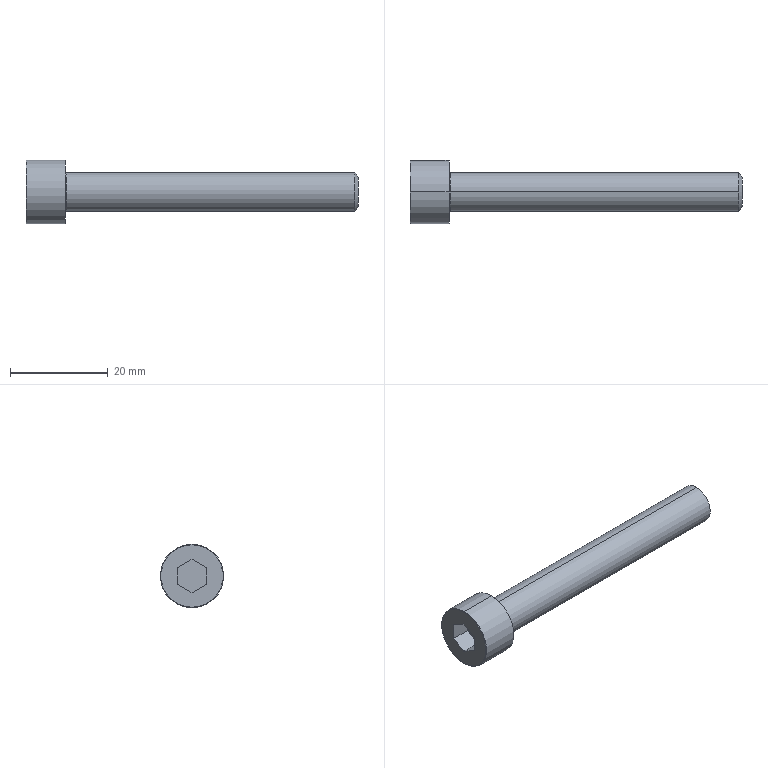Part | STEP file | 1 solid | 20 faces | box 68 x 13 x 13 mm | volume 3948 mm3 | plane 10 | torus 4 | cylinder 4 | cone 2 | commonest cylinder face diameters 8 x2 13 x2
STEP:
#1=CARTESIAN_POINT('',(0.,0.,6.4));
#2=VERTEX_POINT('',#1);
#3=CARTESIAN_POINT('',(0.,0.,-6.4));
#4=VERTEX_POINT('',#3);
#5=CARTESIAN_POINT('',(0.,0.,0.));
#6=DIRECTION('',(-1.,0.,0.));
#7=DIRECTION('',(0.,0.,-1.));
#8=AXIS2_PLACEMENT_3D('',#5,#6,#7);
#9=CIRCLE('',#8,6.4);
#10=EDGE_CURVE('',#2,#4,#9,.T.);
#11=ORIENTED_EDGE('',*,*,#10,.F.);
#12=CARTESIAN_POINT('',(0.1,0.,6.5));
#13=VERTEX_POINT('',#12);
#14=CARTESIAN_POINT('',(0.1,0.,6.4));
#15=DIRECTION('',(0.,1.,0.));
#16=DIRECTION('',(0.,0.,1.));
#17=AXIS2_PLACEMENT_3D('',#14,#15,#16);
#18=CIRCLE('',#17,0.1);
#19=EDGE_CURVE('',#2,#13,#18,.T.);
#20=ORIENTED_EDGE('',*,*,#19,.T.);
#21=CARTESIAN_POINT('',(0.1,0.,-6.5));
#22=VERTEX_POINT('',#21);
#23=CARTESIAN_POINT('',(0.1,0.,0.));
#24=DIRECTION('',(1.,0.,0.));
#25=DIRECTION('',(0.,0.,-1.));
#26=AXIS2_PLACEMENT_3D('',#23,#24,#25);
#27=CIRCLE('',#26,6.5);
#28=EDGE_CURVE('',#22,#13,#27,.T.);
#29=ORIENTED_EDGE('',*,*,#28,.F.);
#30=CARTESIAN_POINT('',(0.1,0.,-6.4));
#31=DIRECTION('',(0.,-1.,0.));
#32=DIRECTION('',(0.,0.,-1.));
#33=AXIS2_PLACEMENT_3D('',#30,#31,#32);
#34=CIRCLE('',#33,0.1);
#35=EDGE_CURVE('',#4,#22,#34,.T.);
#36=ORIENTED_EDGE('',*,*,#35,.F.);
#37=EDGE_LOOP('',(#11,#20,#29,#36));
#38=FACE_OUTER_BOUND('',#37,.T.);
#39=CARTESIAN_POINT('',(0.1,0.,0.));
#40=DIRECTION('',(1.,0.,0.));
#41=DIRECTION('',(0.,0.,-1.));
#42=AXIS2_PLACEMENT_3D('',#39,#40,#41);
#43=TOROIDAL_SURFACE('',#42,6.4,0.1);
#44=ADVANCED_FACE('',(#38),#43,.T.);
#45=CARTESIAN_POINT('',(68.,0.,2.917));
#46=VERTEX_POINT('',#45);
#47=CARTESIAN_POINT('',(68.,0.,-2.917));
#48=VERTEX_POINT('',#47);
#49=CARTESIAN_POINT('',(68.,0.,0.));
#50=DIRECTION('',(-1.,0.,0.));
#51=DIRECTION('',(0.,0.,1.));
#52=AXIS2_PLACEMENT_3D('',#49,#50,#51);
#53=CIRCLE('',#52,2.917);
#54=EDGE_CURVE('',#46,#48,#53,.T.);
#55=ORIENTED_EDGE('',*,*,#54,.T.);
#56=CARTESIAN_POINT('',(67.375,0.,-4.));
#57=VERTEX_POINT('',#56);
#58=CARTESIAN_POINT('',(67.375,0.,-4.));
#59=DIRECTION('',(-0.5,0.,-0.866));
#60=VECTOR('',#59,1000.);
#61=LINE('',#58,#60);
#62=EDGE_CURVE('',#48,#57,#61,.T.);
#63=ORIENTED_EDGE('',*,*,#62,.T.);
#64=CARTESIAN_POINT('',(67.375,0.,4.));
#65=VERTEX_POINT('',#64);
#66=CARTESIAN_POINT('',(67.375,0.,0.));
#67=DIRECTION('',(-1.,0.,0.));
#68=DIRECTION('',(0.,0.,1.));
#69=AXIS2_PLACEMENT_3D('',#66,#67,#68);
#70=CIRCLE('',#69,4.);
#71=EDGE_CURVE('',#65,#57,#70,.T.);
#72=ORIENTED_EDGE('',*,*,#71,.F.);
#73=CARTESIAN_POINT('',(67.375,0.,4.));
#74=DIRECTION('',(-0.5,0.,0.866));
#75=VECTOR('',#74,1000.);
#76=LINE('',#73,#75);
#77=EDGE_CURVE('',#46,#65,#76,.T.);
#78=ORIENTED_EDGE('',*,*,#77,.F.);
#79=EDGE_LOOP('',(#55,#63,#72,#78));
#80=FACE_OUTER_BOUND('',#79,.T.);
#81=CARTESIAN_POINT('',(67.375,0.,0.));
#82=DIRECTION('',(-1.,0.,0.));
#83=DIRECTION('',(0.,0.,1.));
#84=AXIS2_PLACEMENT_3D('',#81,#82,#83);
#85=CONICAL_SURFACE('',#84,4.,1.047);
#86=ADVANCED_FACE('',(#80),#85,.T.);
#87=CARTESIAN_POINT('',(8.,0.,-4.2));
#88=VERTEX_POINT('',#87);
#89=CARTESIAN_POINT('',(8.,0.,4.2));
#90=VERTEX_POINT('',#89);
#91=CARTESIAN_POINT('',(8.,0.,0.));
#92=DIRECTION('',(-1.,0.,0.));
#93=DIRECTION('',(0.,0.,1.));
#94=AXIS2_PLACEMENT_3D('',#91,#92,#93);
#95=CIRCLE('',#94,4.2);
#96=EDGE_CURVE('',#88,#90,#95,.T.);
#97=ORIENTED_EDGE('',*,*,#96,.F.);
#98=CARTESIAN_POINT('',(8.2,0.,-4.));
#99=VERTEX_POINT('',#98);
#100=CARTESIAN_POINT('',(8.2,0.,-4.2));
#101=DIRECTION('',(0.,1.,0.));
#102=DIRECTION('',(0.,0.,1.));
#103=AXIS2_PLACEMENT_3D('',#100,#101,#102);
#104=CIRCLE('',#103,0.2);
#105=EDGE_CURVE('',#88,#99,#104,.T.);
#106=ORIENTED_EDGE('',*,*,#105,.T.);
#107=CARTESIAN_POINT('',(8.2,0.,4.));
#108=VERTEX_POINT('',#107);
#109=CARTESIAN_POINT('',(8.2,0.,0.));
#110=DIRECTION('',(-1.,0.,0.));
#111=DIRECTION('',(0.,0.,1.));
#112=AXIS2_PLACEMENT_3D('',#109,#110,#111);
#113=CIRCLE('',#112,4.);
#114=EDGE_CURVE('',#99,#108,#113,.T.);
#115=ORIENTED_EDGE('',*,*,#114,.T.);
#116=CARTESIAN_POINT('',(8.2,0.,4.2));
#117=DIRECTION('',(0.,-1.,0.));
#118=DIRECTION('',(0.,0.,-1.));
#119=AXIS2_PLACEMENT_3D('',#116,#117,#118);
#120=CIRCLE('',#119,0.2);
#121=EDGE_CURVE('',#90,#108,#120,.T.);
#122=ORIENTED_EDGE('',*,*,#121,.F.);
#123=EDGE_LOOP('',(#97,#106,#115,#122));
#124=FACE_OUTER_BOUND('',#123,.T.);
#125=CARTESIAN_POINT('',(8.2,0.,0.));
#126=DIRECTION('',(-1.,0.,0.));
#127=DIRECTION('',(0.,0.,1.));
#128=AXIS2_PLACEMENT_3D('',#125,#126,#127);
#129=TOROIDAL_SURFACE('',#128,4.2,0.2);
#130=ADVANCED_FACE('',(#124),#129,.F.);
#131=CARTESIAN_POINT('',(8.,0.,6.5));
#132=VERTEX_POINT('',#131);
#133=CARTESIAN_POINT('',(8.,0.,-6.5));
#134=VERTEX_POINT('',#133);
#135=CARTESIAN_POINT('',(8.,0.,0.));
#136=DIRECTION('',(-1.,0.,0.));
#137=DIRECTION('',(0.,0.,1.));
#138=AXIS2_PLACEMENT_3D('',#135,#136,#137);
#139=CIRCLE('',#138,6.5);
#140=EDGE_CURVE('',#132,#134,#139,.T.);
#141=ORIENTED_EDGE('',*,*,#140,.T.);
#142=CARTESIAN_POINT('',(0.,0.,-6.5));
#143=DIRECTION('',(-1.,0.,0.));
#144=VECTOR('',#143,1000.);
#145=LINE('',#142,#144);
#146=EDGE_CURVE('',#134,#22,#145,.T.);
#147=ORIENTED_EDGE('',*,*,#146,.T.);
#148=ORIENTED_EDGE('',*,*,#28,.T.);
#149=CARTESIAN_POINT('',(0.,0.,6.5));
#150=DIRECTION('',(-1.,0.,0.));
#151=VECTOR('',#150,1000.);
#152=LINE('',#149,#151);
#153=EDGE_CURVE('',#132,#13,#152,.T.);
#154=ORIENTED_EDGE('',*,*,#153,.F.);
#155=EDGE_LOOP('',(#141,#147,#148,#154));
#156=FACE_OUTER_BOUND('',#155,.T.);
#157=CARTESIAN_POINT('',(0.,0.,0.));
#158=DIRECTION('',(-1.,0.,0.));
#159=DIRECTION('',(0.,0.,1.));
#160=AXIS2_PLACEMENT_3D('',#157,#158,#159);
#161=CYLINDRICAL_SURFACE('',#160,6.5);
#162=ADVANCED_FACE('',(#156),#161,.T.);
#163=ORIENTED_EDGE('',*,*,#71,.T.);
#164=CARTESIAN_POINT('',(0.,0.,-4.));
#165=DIRECTION('',(-1.,0.,0.));
#166=VECTOR('',#165,1000.);
#167=LINE('',#164,#166);
#168=EDGE_CURVE('',#57,#99,#167,.T.);
#169=ORIENTED_EDGE('',*,*,#168,.T.);
#170=CARTESIAN_POINT('',(8.2,0.,0.));
#171=DIRECTION('',(-1.,0.,0.));
#172=DIRECTION('',(0.,0.,1.));
#173=AXIS2_PLACEMENT_3D('',#170,#171,#172);
#174=CIRCLE('',#173,4.);
#175=EDGE_CURVE('',#108,#99,#174,.T.);
#176=ORIENTED_EDGE('',*,*,#175,.F.);
#177=CARTESIAN_POINT('',(0.,0.,4.));
#178=DIRECTION('',(-1.,0.,0.));
#179=VECTOR('',#178,1000.);
#180=LINE('',#177,#179);
#181=EDGE_CURVE('',#65,#108,#180,.T.);
#182=ORIENTED_EDGE('',*,*,#181,.F.);
#183=EDGE_LOOP('',(#163,#169,#176,#182));
#184=FACE_OUTER_BOUND('',#183,.T.);
#185=CARTESIAN_POINT('',(0.,0.,0.));
#186=DIRECTION('',(-1.,0.,0.));
#187=DIRECTION('',(0.,0.,1.));
#188=AXIS2_PLACEMENT_3D('',#185,#186,#187);
#189=CYLINDRICAL_SURFACE('',#188,4.);
#190=ADVANCED_FACE('',(#184),#189,.T.);
#191=ORIENTED_EDGE('',*,*,#168,.F.);
#192=CARTESIAN_POINT('',(67.375,0.,0.));
#193=DIRECTION('',(-1.,0.,0.));
#194=DIRECTION('',(0.,0.,1.));
#195=AXIS2_PLACEMENT_3D('',#192,#193,#194);
#196=CIRCLE('',#195,4.);
#197=EDGE_CURVE('',#57,#65,#196,.T.);
#198=ORIENTED_EDGE('',*,*,#197,.T.);
#199=ORIENTED_EDGE('',*,*,#181,.T.);
#200=ORIENTED_EDGE('',*,*,#114,.F.);
#201=EDGE_LOOP('',(#191,#198,#199,#200));
#202=FACE_OUTER_BOUND('',#201,.T.);
#203=CARTESIAN_POINT('',(0.,0.,0.));
#204=DIRECTION('',(-1.,0.,0.));
#205=DIRECTION('',(0.,0.,1.));
#206=AXIS2_PLACEMENT_3D('',#203,#204,#205);
#207=CYLINDRICAL_SURFACE('',#206,4.);
#208=ADVANCED_FACE('',(#202),#207,.T.);
#209=CARTESIAN_POINT('',(0.,0.,0.));
#210=DIRECTION('',(-1.,0.,0.));
#211=DIRECTION('',(0.,0.,-1.));
#212=AXIS2_PLACEMENT_3D('',#209,#210,#211);
#213=CIRCLE('',#212,6.4);
#214=EDGE_CURVE('',#4,#2,#213,.T.);
#215=ORIENTED_EDGE('',*,*,#214,.T.);
#216=ORIENTED_EDGE('',*,*,#10,.T.);
#217=EDGE_LOOP('',(#215,#216));
#218=FACE_OUTER_BOUND('',#217,.T.);
#219=CARTESIAN_POINT('',(0.,0.,3.43));
#220=VERTEX_POINT('',#219);
#221=CARTESIAN_POINT('',(0.,2.97,1.715));
#222=VERTEX_POINT('',#221);
#223=CARTESIAN_POINT('',(0.,0.,3.43));
#224=DIRECTION('',(0.,0.866,-0.5));
#225=VECTOR('',#224,1000.);
#226=LINE('',#223,#225);
#227=EDGE_CURVE('',#220,#222,#226,.T.);
#228=ORIENTED_EDGE('',*,*,#227,.F.);
#229=CARTESIAN_POINT('',(0.,-2.97,1.715));
#230=VERTEX_POINT('',#229);
#231=CARTESIAN_POINT('',(0.,-2.97,1.715));
#232=DIRECTION('',(0.,0.866,0.5));
#233=VECTOR('',#232,1000.);
#234=LINE('',#231,#233);
#235=EDGE_CURVE('',#230,#220,#234,.T.);
#236=ORIENTED_EDGE('',*,*,#235,.F.);
#237=CARTESIAN_POINT('',(0.,-2.97,-1.715));
#238=VERTEX_POINT('',#237);
#239=CARTESIAN_POINT('',(0.,-2.97,-1.715));
#240=DIRECTION('',(0.,0.,1.));
#241=VECTOR('',#240,1000.);
#242=LINE('',#239,#241);
#243=EDGE_CURVE('',#238,#230,#242,.T.);
#244=ORIENTED_EDGE('',*,*,#243,.F.);
#245=CARTESIAN_POINT('',(0.,0.,-3.43));
#246=VERTEX_POINT('',#245);
#247=CARTESIAN_POINT('',(0.,0.,-3.43));
#248=DIRECTION('',(0.,-0.866,0.5));
#249=VECTOR('',#248,1000.);
#250=LINE('',#247,#249);
#251=EDGE_CURVE('',#246,#238,#250,.T.);
#252=ORIENTED_EDGE('',*,*,#251,.F.);
#253=CARTESIAN_POINT('',(0.,2.97,-1.715));
#254=VERTEX_POINT('',#253);
#255=CARTESIAN_POINT('',(0.,2.97,-1.715));
#256=DIRECTION('',(0.,-0.866,-0.5));
#257=VECTOR('',#256,1000.);
#258=LINE('',#255,#257);
#259=EDGE_CURVE('',#254,#246,#258,.T.);
#260=ORIENTED_EDGE('',*,*,#259,.F.);
#261=CARTESIAN_POINT('',(0.,2.97,1.715));
#262=DIRECTION('',(0.,0.,-1.));
#263=VECTOR('',#262,1000.);
#264=LINE('',#261,#263);
#265=EDGE_CURVE('',#222,#254,#264,.T.);
#266=ORIENTED_EDGE('',*,*,#265,.F.);
#267=EDGE_LOOP('',(#228,#236,#244,#252,#260,#266));
#268=FACE_BOUND('',#267,.T.);
#269=CARTESIAN_POINT('',(0.,0.,0.));
#270=DIRECTION('',(1.,0.,0.));
#271=DIRECTION('',(0.,0.,-1.));
#272=AXIS2_PLACEMENT_3D('',#269,#270,#271);
#273=PLANE('',#272);
#274=ADVANCED_FACE('',(#218,#268),#273,.F.);
#275=ORIENTED_EDGE('',*,*,#146,.F.);
#276=CARTESIAN_POINT('',(8.,0.,0.));
#277=DIRECTION('',(-1.,0.,0.));
#278=DIRECTION('',(0.,0.,1.));
#279=AXIS2_PLACEMENT_3D('',#276,#277,#278);
#280=CIRCLE('',#279,6.5);
#281=EDGE_CURVE('',#134,#132,#280,.T.);
#282=ORIENTED_EDGE('',*,*,#281,.T.);
#283=ORIENTED_EDGE('',*,*,#153,.T.);
#284=CARTESIAN_POINT('',(0.1,0.,0.));
#285=DIRECTION('',(1.,0.,0.));
#286=DIRECTION('',(0.,0.,-1.));
#287=AXIS2_PLACEMENT_3D('',#284,#285,#286);
#288=CIRCLE('',#287,6.5);
#289=EDGE_CURVE('',#13,#22,#288,.T.);
#290=ORIENTED_EDGE('',*,*,#289,.T.);
#291=EDGE_LOOP('',(#275,#282,#283,#290));
#292=FACE_OUTER_BOUND('',#291,.T.);
#293=CARTESIAN_POINT('',(0.,0.,0.));
#294=DIRECTION('',(-1.,0.,0.));
#295=DIRECTION('',(0.,0.,1.));
#296=AXIS2_PLACEMENT_3D('',#293,#294,#295);
#297=CYLINDRICAL_SURFACE('',#296,6.5);
#298=ADVANCED_FACE('',(#292),#297,.T.);
#299=ORIENTED_EDGE('',*,*,#140,.F.);
#300=ORIENTED_EDGE('',*,*,#281,.F.);
#301=EDGE_LOOP('',(#299,#300));
#302=FACE_OUTER_BOUND('',#301,.T.);
#303=CARTESIAN_POINT('',(8.,0.,0.));
#304=DIRECTION('',(-1.,0.,0.));
#305=DIRECTION('',(0.,0.,1.));
#306=AXIS2_PLACEMENT_3D('',#303,#304,#305);
#307=CIRCLE('',#306,4.2);
#308=EDGE_CURVE('',#90,#88,#307,.T.);
#309=ORIENTED_EDGE('',*,*,#308,.T.);
#310=ORIENTED_EDGE('',*,*,#96,.T.);
#311=EDGE_LOOP('',(#309,#310));
#312=FACE_BOUND('',#311,.T.);
#313=CARTESIAN_POINT('',(8.,6.5,0.));
#314=DIRECTION('',(-1.,0.,0.));
#315=DIRECTION('',(0.,0.,1.));
#316=AXIS2_PLACEMENT_3D('',#313,#314,#315);
#317=PLANE('',#316);
#318=ADVANCED_FACE('',(#302,#312),#317,.F.);
#319=ORIENTED_EDGE('',*,*,#105,.F.);
#320=ORIENTED_EDGE('',*,*,#308,.F.);
#321=ORIENTED_EDGE('',*,*,#121,.T.);
#322=ORIENTED_EDGE('',*,*,#175,.T.);
#323=EDGE_LOOP('',(#319,#320,#321,#322));
#324=FACE_OUTER_BOUND('',#323,.T.);
#325=CARTESIAN_POINT('',(8.2,0.,0.));
#326=DIRECTION('',(-1.,0.,0.));
#327=DIRECTION('',(0.,0.,1.));
#328=AXIS2_PLACEMENT_3D('',#325,#326,#327);
#329=TOROIDAL_SURFACE('',#328,4.2,0.2);
#330=ADVANCED_FACE('',(#324),#329,.F.);
#331=ORIENTED_EDGE('',*,*,#235,.T.);
#332=CARTESIAN_POINT('',(4.,0.,3.43));
#333=VERTEX_POINT('',#332);
#334=CARTESIAN_POINT('',(4.,0.,3.43));
#335=DIRECTION('',(-1.,0.,0.));
#336=VECTOR('',#335,1000.);
#337=LINE('',#334,#336);
#338=EDGE_CURVE('',#333,#220,#337,.T.);
#339=ORIENTED_EDGE('',*,*,#338,.F.);
#340=CARTESIAN_POINT('',(4.,-2.97,1.715));
#341=VERTEX_POINT('',#340);
#342=CARTESIAN_POINT('',(4.,-2.97,1.715));
#343=DIRECTION('',(0.,0.866,0.5));
#344=VECTOR('',#343,1000.);
#345=LINE('',#342,#344);
#346=EDGE_CURVE('',#341,#333,#345,.T.);
#347=ORIENTED_EDGE('',*,*,#346,.F.);
#348=CARTESIAN_POINT('',(4.,-2.97,1.715));
#349=DIRECTION('',(-1.,0.,0.));
#350=VECTOR('',#349,1000.);
#351=LINE('',#348,#350);
#352=EDGE_CURVE('',#341,#230,#351,.T.);
#353=ORIENTED_EDGE('',*,*,#352,.T.);
#354=EDGE_LOOP('',(#331,#339,#347,#353));
#355=FACE_OUTER_BOUND('',#354,.T.);
#356=CARTESIAN_POINT('',(4.,-2.97,1.715));
#357=DIRECTION('',(0.,-0.5,0.866));
#358=DIRECTION('',(0.,-0.866,-0.5));
#359=AXIS2_PLACEMENT_3D('',#356,#357,#358);
#360=PLANE('',#359);
#361=ADVANCED_FACE('',(#355),#360,.F.);
#362=ORIENTED_EDGE('',*,*,#243,.T.);
#363=ORIENTED_EDGE('',*,*,#352,.F.);
#364=CARTESIAN_POINT('',(4.,-2.97,-1.715));
#365=VERTEX_POINT('',#364);
#366=CARTESIAN_POINT('',(4.,-2.97,-1.715));
#367=DIRECTION('',(0.,0.,1.));
#368=VECTOR('',#367,1000.);
#369=LINE('',#366,#368);
#370=EDGE_CURVE('',#365,#341,#369,.T.);
#371=ORIENTED_EDGE('',*,*,#370,.F.);
#372=CARTESIAN_POINT('',(4.,-2.97,-1.715));
#373=DIRECTION('',(-1.,0.,0.));
#374=VECTOR('',#373,1000.);
#375=LINE('',#372,#374);
#376=EDGE_CURVE('',#365,#238,#375,.T.);
#377=ORIENTED_EDGE('',*,*,#376,.T.);
#378=EDGE_LOOP('',(#362,#363,#371,#377));
#379=FACE_OUTER_BOUND('',#378,.T.);
#380=CARTESIAN_POINT('',(4.,-2.97,-1.715));
#381=DIRECTION('',(0.,-1.,0.));
#382=DIRECTION('',(0.,0.,-1.));
#383=AXIS2_PLACEMENT_3D('',#380,#381,#382);
#384=PLANE('',#383);
#385=ADVANCED_FACE('',(#379),#384,.F.);
#386=ORIENTED_EDGE('',*,*,#251,.T.);
#387=ORIENTED_EDGE('',*,*,#376,.F.);
#388=CARTESIAN_POINT('',(4.,0.,-3.43));
#389=VERTEX_POINT('',#388);
#390=CARTESIAN_POINT('',(4.,0.,-3.43));
#391=DIRECTION('',(0.,-0.866,0.5));
#392=VECTOR('',#391,1000.);
#393=LINE('',#390,#392);
#394=EDGE_CURVE('',#389,#365,#393,.T.);
#395=ORIENTED_EDGE('',*,*,#394,.F.);
#396=CARTESIAN_POINT('',(4.,0.,-3.43));
#397=DIRECTION('',(-1.,0.,0.));
#398=VECTOR('',#397,1000.);
#399=LINE('',#396,#398);
#400=EDGE_CURVE('',#389,#246,#399,.T.);
#401=ORIENTED_EDGE('',*,*,#400,.T.);
#402=EDGE_LOOP('',(#386,#387,#395,#401));
#403=FACE_OUTER_BOUND('',#402,.T.);
#404=CARTESIAN_POINT('',(4.,0.,-3.43));
#405=DIRECTION('',(0.,-0.5,-0.866));
#406=DIRECTION('',(0.,0.866,-0.5));
#407=AXIS2_PLACEMENT_3D('',#404,#405,#406);
#408=PLANE('',#407);
#409=ADVANCED_FACE('',(#403),#408,.F.);
#410=ORIENTED_EDGE('',*,*,#259,.T.);
#411=ORIENTED_EDGE('',*,*,#400,.F.);
#412=CARTESIAN_POINT('',(4.,2.97,-1.715));
#413=VERTEX_POINT('',#412);
#414=CARTESIAN_POINT('',(4.,2.97,-1.715));
#415=DIRECTION('',(0.,-0.866,-0.5));
#416=VECTOR('',#415,1000.);
#417=LINE('',#414,#416);
#418=EDGE_CURVE('',#413,#389,#417,.T.);
#419=ORIENTED_EDGE('',*,*,#418,.F.);
#420=CARTESIAN_POINT('',(4.,2.97,-1.715));
#421=DIRECTION('',(-1.,0.,0.));
#422=VECTOR('',#421,1000.);
#423=LINE('',#420,#422);
#424=EDGE_CURVE('',#413,#254,#423,.T.);
#425=ORIENTED_EDGE('',*,*,#424,.T.);
#426=EDGE_LOOP('',(#410,#411,#419,#425));
#427=FACE_OUTER_BOUND('',#426,.T.);
#428=CARTESIAN_POINT('',(4.,2.97,-1.715));
#429=DIRECTION('',(0.,0.5,-0.866));
#430=DIRECTION('',(0.,0.866,0.5));
#431=AXIS2_PLACEMENT_3D('',#428,#429,#430);
#432=PLANE('',#431);
#433=ADVANCED_FACE('',(#427),#432,.F.);
#434=ORIENTED_EDGE('',*,*,#265,.T.);
#435=ORIENTED_EDGE('',*,*,#424,.F.);
#436=CARTESIAN_POINT('',(4.,2.97,1.715));
#437=VERTEX_POINT('',#436);
#438=CARTESIAN_POINT('',(4.,2.97,1.715));
#439=DIRECTION('',(0.,0.,-1.));
#440=VECTOR('',#439,1000.);
#441=LINE('',#438,#440);
#442=EDGE_CURVE('',#437,#413,#441,.T.);
#443=ORIENTED_EDGE('',*,*,#442,.F.);
#444=CARTESIAN_POINT('',(4.,2.97,1.715));
#445=DIRECTION('',(-1.,0.,0.));
#446=VECTOR('',#445,1000.);
#447=LINE('',#444,#446);
#448=EDGE_CURVE('',#437,#222,#447,.T.);
#449=ORIENTED_EDGE('',*,*,#448,.T.);
#450=EDGE_LOOP('',(#434,#435,#443,#449));
#451=FACE_OUTER_BOUND('',#450,.T.);
#452=CARTESIAN_POINT('',(4.,2.97,1.715));
#453=DIRECTION('',(0.,1.,0.));
#454=DIRECTION('',(0.,0.,1.));
#455=AXIS2_PLACEMENT_3D('',#452,#453,#454);
#456=PLANE('',#455);
#457=ADVANCED_FACE('',(#451),#456,.F.);
#458=ORIENTED_EDGE('',*,*,#227,.T.);
#459=ORIENTED_EDGE('',*,*,#448,.F.);
#460=CARTESIAN_POINT('',(4.,0.,3.43));
#461=DIRECTION('',(0.,0.866,-0.5));
#462=VECTOR('',#461,1000.);
#463=LINE('',#460,#462);
#464=EDGE_CURVE('',#333,#437,#463,.T.);
#465=ORIENTED_EDGE('',*,*,#464,.F.);
#466=ORIENTED_EDGE('',*,*,#338,.T.);
#467=EDGE_LOOP('',(#458,#459,#465,#466));
#468=FACE_OUTER_BOUND('',#467,.T.);
#469=CARTESIAN_POINT('',(4.,0.,3.43));
#470=DIRECTION('',(0.,0.5,0.866));
#471=DIRECTION('',(0.,-0.866,0.5));
#472=AXIS2_PLACEMENT_3D('',#469,#470,#471);
#473=PLANE('',#472);
#474=ADVANCED_FACE('',(#468),#473,.F.);
#475=ORIENTED_EDGE('',*,*,#346,.T.);
#476=ORIENTED_EDGE('',*,*,#464,.T.);
#477=ORIENTED_EDGE('',*,*,#442,.T.);
#478=ORIENTED_EDGE('',*,*,#418,.T.);
#479=ORIENTED_EDGE('',*,*,#394,.T.);
#480=ORIENTED_EDGE('',*,*,#370,.T.);
#481=EDGE_LOOP('',(#475,#476,#477,#478,#479,#480));
#482=FACE_OUTER_BOUND('',#481,.T.);
#483=CARTESIAN_POINT('',(4.,-2.97,1.715));
#484=DIRECTION('',(1.,0.,0.));
#485=DIRECTION('',(0.,0.,-1.));
#486=AXIS2_PLACEMENT_3D('',#483,#484,#485);
#487=PLANE('',#486);
#488=ADVANCED_FACE('',(#482),#487,.F.);
#489=ORIENTED_EDGE('',*,*,#62,.F.);
#490=CARTESIAN_POINT('',(68.,0.,0.));
#491=DIRECTION('',(-1.,0.,0.));
#492=DIRECTION('',(0.,0.,1.));
#493=AXIS2_PLACEMENT_3D('',#490,#491,#492);
#494=CIRCLE('',#493,2.917);
#495=EDGE_CURVE('',#48,#46,#494,.T.);
#496=ORIENTED_EDGE('',*,*,#495,.T.);
#497=ORIENTED_EDGE('',*,*,#77,.T.);
#498=ORIENTED_EDGE('',*,*,#197,.F.);
#499=EDGE_LOOP('',(#489,#496,#497,#498));
#500=FACE_OUTER_BOUND('',#499,.T.);
#501=CARTESIAN_POINT('',(67.375,0.,0.));
#502=DIRECTION('',(-1.,0.,0.));
#503=DIRECTION('',(0.,0.,1.));
#504=AXIS2_PLACEMENT_3D('',#501,#502,#503);
#505=CONICAL_SURFACE('',#504,4.,1.047);
#506=ADVANCED_FACE('',(#500),#505,.T.);
#507=ORIENTED_EDGE('',*,*,#54,.F.);
#508=ORIENTED_EDGE('',*,*,#495,.F.);
#509=EDGE_LOOP('',(#507,#508));
#510=FACE_OUTER_BOUND('',#509,.T.);
#511=CARTESIAN_POINT('',(68.,4.,0.));
#512=DIRECTION('',(-1.,0.,0.));
#513=DIRECTION('',(0.,0.,1.));
#514=AXIS2_PLACEMENT_3D('',#511,#512,#513);
#515=PLANE('',#514);
#516=ADVANCED_FACE('',(#510),#515,.F.);
#517=ORIENTED_EDGE('',*,*,#19,.F.);
#518=ORIENTED_EDGE('',*,*,#214,.F.);
#519=ORIENTED_EDGE('',*,*,#35,.T.);
#520=ORIENTED_EDGE('',*,*,#289,.F.);
#521=EDGE_LOOP('',(#517,#518,#519,#520));
#522=FACE_OUTER_BOUND('',#521,.T.);
#523=CARTESIAN_POINT('',(0.1,0.,0.));
#524=DIRECTION('',(1.,0.,0.));
#525=DIRECTION('',(0.,0.,-1.));
#526=AXIS2_PLACEMENT_3D('',#523,#524,#525);
#527=TOROIDAL_SURFACE('',#526,6.4,0.1);
#528=ADVANCED_FACE('',(#522),#527,.T.);
#529=CLOSED_SHELL('',(#44,#86,#130,#162,#190,#208,#274,#298,#318,#330,#361,#385,#409,#433,#457,#474,#488,#506,#516,#528));
#530=MANIFOLD_SOLID_BREP('',#529);
#531=CARTESIAN_POINT('',(0.,0.,0.));
#532=DIRECTION('',(0.,0.,1.));
#533=DIRECTION('',(1.,0.,0.));
#534=AXIS2_PLACEMENT_3D('',#531,#532,#533);
#535=(LENGTH_UNIT()NAMED_UNIT(*)SI_UNIT(.MILLI.,.METRE.));
#536=UNCERTAINTY_MEASURE_WITH_UNIT(LENGTH_MEASURE(0.00001),#535,'','');
#537=(NAMED_UNIT(*)PLANE_ANGLE_UNIT()SI_UNIT($,.RADIAN.));
#538=(NAMED_UNIT(*)SI_UNIT($,.STERADIAN.)SOLID_ANGLE_UNIT());
#539=(GEOMETRIC_REPRESENTATION_CONTEXT(3)GLOBAL_UNCERTAINTY_ASSIGNED_CONTEXT((#536))GLOBAL_UNIT_ASSIGNED_CONTEXT((#535,#537,#538))REPRESENTATION_CONTEXT('',''));
#540=ADVANCED_BREP_SHAPE_REPRESENTATION('',(#530,#534),#539);